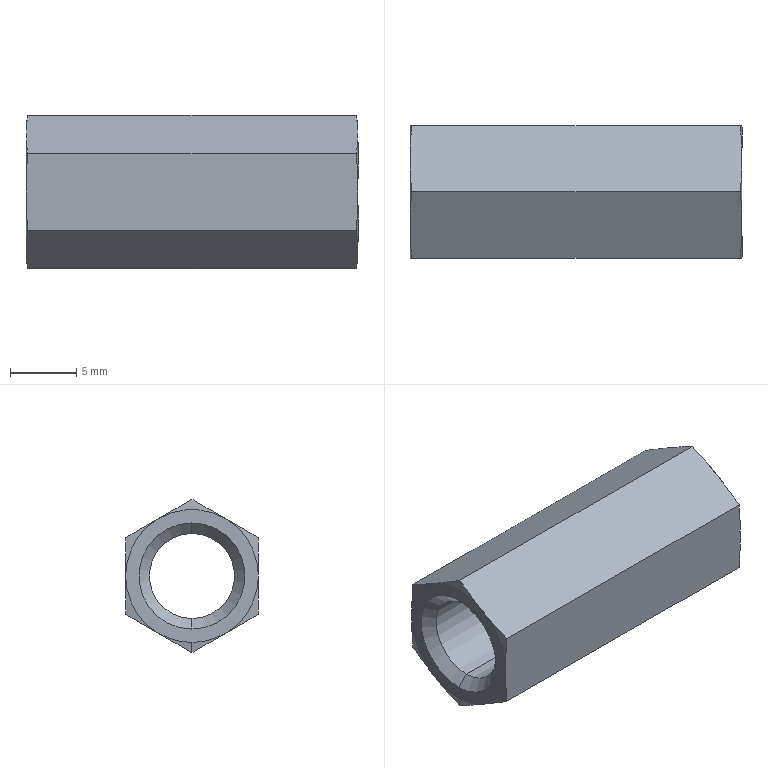Part | STEP file | 1 solid | 28 faces | box 25 x 10 x 11.547 mm | volume 1346 mm3 | cone 18 | plane 8 | cylinder 2 | commonest cylinder face diameters 6.4 x2